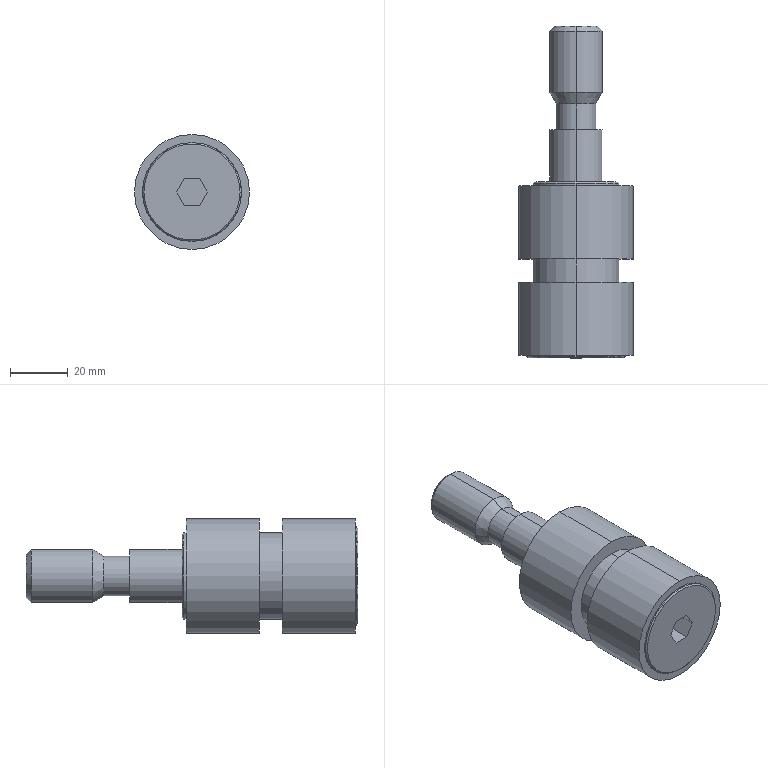Part | SolidWorks | features BaseBody 1 | 1 solid | 39 faces | box 40 x 115.385 x 40 mm | volume 83771 mm3 | cylinder 16 | plane 15 | cone 8 | commonest cylinder face diameters 18.462 x4 30 x4 40 x4 13.846 x2 34.385 x2
STEP:
#1=CARTESIAN_POINT('',(57.247,271.192,266.154));
#2=VERTEX_POINT('',#1);
#3=CARTESIAN_POINT('',(57.247,271.192,226.154));
#4=VERTEX_POINT('',#3);
#5=CARTESIAN_POINT('',(57.247,271.192,246.154));
#6=DIRECTION('',(0.,1.,0.));
#7=DIRECTION('',(0.,0.,1.));
#8=AXIS2_PLACEMENT_3D('',#5,#6,#7);
#9=CIRCLE('',#8,20.);
#10=EDGE_CURVE('',#2,#4,#9,.T.);
#11=ORIENTED_EDGE('',*,*,#10,.T.);
#12=CARTESIAN_POINT('',(57.247,296.577,226.154));
#13=VERTEX_POINT('',#12);
#14=CARTESIAN_POINT('',(57.247,270.269,226.154));
#15=DIRECTION('',(0.,1.,0.));
#16=VECTOR('',#15,1000.);
#17=LINE('',#14,#16);
#18=EDGE_CURVE('',#4,#13,#17,.T.);
#19=ORIENTED_EDGE('',*,*,#18,.T.);
#20=CARTESIAN_POINT('',(57.247,296.577,266.154));
#21=VERTEX_POINT('',#20);
#22=CARTESIAN_POINT('',(57.247,296.577,246.154));
#23=DIRECTION('',(0.,-1.,0.));
#24=DIRECTION('',(0.,0.,1.));
#25=AXIS2_PLACEMENT_3D('',#22,#23,#24);
#26=CIRCLE('',#25,20.);
#27=EDGE_CURVE('',#13,#21,#26,.T.);
#28=ORIENTED_EDGE('',*,*,#27,.T.);
#29=CARTESIAN_POINT('',(57.247,270.269,266.154));
#30=DIRECTION('',(0.,1.,0.));
#31=VECTOR('',#30,1000.);
#32=LINE('',#29,#31);
#33=EDGE_CURVE('',#2,#21,#32,.T.);
#34=ORIENTED_EDGE('',*,*,#33,.F.);
#35=EDGE_LOOP('',(#11,#19,#28,#34));
#36=FACE_OUTER_BOUND('',#35,.T.);
#37=CARTESIAN_POINT('',(57.247,270.269,246.154));
#38=DIRECTION('',(0.,1.,0.));
#39=DIRECTION('',(0.,0.,1.));
#40=AXIS2_PLACEMENT_3D('',#37,#38,#39);
#41=CYLINDRICAL_SURFACE('',#40,20.);
#42=ADVANCED_FACE('',(#36),#41,.T.);
#43=CARTESIAN_POINT('',(74.439,270.731,246.154));
#44=VERTEX_POINT('',#43);
#45=CARTESIAN_POINT('',(57.247,270.731,228.962));
#46=VERTEX_POINT('',#45);
#47=CARTESIAN_POINT('',(57.247,270.731,246.154));
#48=DIRECTION('',(0.,1.,0.));
#49=DIRECTION('',(0.,0.,1.));
#50=AXIS2_PLACEMENT_3D('',#47,#48,#49);
#51=CIRCLE('',#50,17.192);
#52=EDGE_CURVE('',#44,#46,#51,.T.);
#53=ORIENTED_EDGE('',*,*,#52,.T.);
#54=CARTESIAN_POINT('',(57.247,271.192,228.962));
#55=VERTEX_POINT('',#54);
#56=CARTESIAN_POINT('',(57.247,270.269,228.962));
#57=DIRECTION('',(0.,1.,0.));
#58=VECTOR('',#57,1000.);
#59=LINE('',#56,#58);
#60=EDGE_CURVE('',#46,#55,#59,.T.);
#61=ORIENTED_EDGE('',*,*,#60,.T.);
#62=CARTESIAN_POINT('',(57.247,271.192,263.346));
#63=VERTEX_POINT('',#62);
#64=CARTESIAN_POINT('',(57.247,271.192,246.154));
#65=DIRECTION('',(0.,-1.,0.));
#66=DIRECTION('',(0.,0.,1.));
#67=AXIS2_PLACEMENT_3D('',#64,#65,#66);
#68=CIRCLE('',#67,17.192);
#69=EDGE_CURVE('',#55,#63,#68,.T.);
#70=ORIENTED_EDGE('',*,*,#69,.T.);
#71=CARTESIAN_POINT('',(57.247,270.731,263.346));
#72=VERTEX_POINT('',#71);
#73=CARTESIAN_POINT('',(57.247,270.269,263.346));
#74=DIRECTION('',(0.,1.,0.));
#75=VECTOR('',#74,1000.);
#76=LINE('',#73,#75);
#77=EDGE_CURVE('',#72,#63,#76,.T.);
#78=ORIENTED_EDGE('',*,*,#77,.F.);
#79=CARTESIAN_POINT('',(57.247,270.731,246.154));
#80=DIRECTION('',(0.,1.,0.));
#81=DIRECTION('',(0.,0.,1.));
#82=AXIS2_PLACEMENT_3D('',#79,#80,#81);
#83=CIRCLE('',#82,17.192);
#84=EDGE_CURVE('',#72,#44,#83,.T.);
#85=ORIENTED_EDGE('',*,*,#84,.T.);
#86=EDGE_LOOP('',(#53,#61,#70,#78,#85));
#87=FACE_OUTER_BOUND('',#86,.T.);
#88=CARTESIAN_POINT('',(57.247,270.269,246.154));
#89=DIRECTION('',(0.,1.,0.));
#90=DIRECTION('',(0.,0.,1.));
#91=AXIS2_PLACEMENT_3D('',#88,#89,#90);
#92=CYLINDRICAL_SURFACE('',#91,17.192);
#93=ADVANCED_FACE('',(#87),#92,.T.);
#94=CARTESIAN_POINT('',(57.247,296.577,261.154));
#95=VERTEX_POINT('',#94);
#96=CARTESIAN_POINT('',(57.247,296.577,231.154));
#97=VERTEX_POINT('',#96);
#98=CARTESIAN_POINT('',(57.247,296.577,246.154));
#99=DIRECTION('',(0.,1.,0.));
#100=DIRECTION('',(0.,0.,1.));
#101=AXIS2_PLACEMENT_3D('',#98,#99,#100);
#102=CIRCLE('',#101,15.);
#103=EDGE_CURVE('',#95,#97,#102,.T.);
#104=ORIENTED_EDGE('',*,*,#103,.T.);
#105=CARTESIAN_POINT('',(57.247,304.654,231.154));
#106=VERTEX_POINT('',#105);
#107=CARTESIAN_POINT('',(57.247,270.269,231.154));
#108=DIRECTION('',(0.,1.,0.));
#109=VECTOR('',#108,1000.);
#110=LINE('',#107,#109);
#111=EDGE_CURVE('',#97,#106,#110,.T.);
#112=ORIENTED_EDGE('',*,*,#111,.T.);
#113=CARTESIAN_POINT('',(57.247,304.654,261.154));
#114=VERTEX_POINT('',#113);
#115=CARTESIAN_POINT('',(57.247,304.654,246.154));
#116=DIRECTION('',(0.,-1.,0.));
#117=DIRECTION('',(0.,0.,1.));
#118=AXIS2_PLACEMENT_3D('',#115,#116,#117);
#119=CIRCLE('',#118,15.);
#120=EDGE_CURVE('',#106,#114,#119,.T.);
#121=ORIENTED_EDGE('',*,*,#120,.T.);
#122=CARTESIAN_POINT('',(57.247,270.269,261.154));
#123=DIRECTION('',(0.,1.,0.));
#124=VECTOR('',#123,1000.);
#125=LINE('',#122,#124);
#126=EDGE_CURVE('',#95,#114,#125,.T.);
#127=ORIENTED_EDGE('',*,*,#126,.F.);
#128=EDGE_LOOP('',(#104,#112,#121,#127));
#129=FACE_OUTER_BOUND('',#128,.T.);
#130=CARTESIAN_POINT('',(57.247,270.269,246.154));
#131=DIRECTION('',(0.,1.,0.));
#132=DIRECTION('',(0.,0.,1.));
#133=AXIS2_PLACEMENT_3D('',#130,#131,#132);
#134=CYLINDRICAL_SURFACE('',#133,15.);
#135=ADVANCED_FACE('',(#129),#134,.T.);
#136=CARTESIAN_POINT('',(40.516,270.269,246.154));
#137=VERTEX_POINT('',#136);
#138=CARTESIAN_POINT('',(73.977,270.269,246.154));
#139=VERTEX_POINT('',#138);
#140=CARTESIAN_POINT('',(57.247,270.269,246.154));
#141=DIRECTION('',(0.,1.,0.));
#142=DIRECTION('',(-1.,0.,0.));
#143=AXIS2_PLACEMENT_3D('',#140,#141,#142);
#144=CIRCLE('',#143,16.731);
#145=EDGE_CURVE('',#137,#139,#144,.T.);
#146=ORIENTED_EDGE('',*,*,#145,.T.);
#147=CARTESIAN_POINT('',(74.439,270.731,246.154));
#148=DIRECTION('',(0.7071,0.7071,0.));
#149=VECTOR('',#148,1000.);
#150=LINE('',#147,#149);
#151=EDGE_CURVE('',#139,#44,#150,.T.);
#152=ORIENTED_EDGE('',*,*,#151,.T.);
#153=ORIENTED_EDGE('',*,*,#84,.F.);
#154=CARTESIAN_POINT('',(40.054,270.731,246.154));
#155=VERTEX_POINT('',#154);
#156=CARTESIAN_POINT('',(57.247,270.731,246.154));
#157=DIRECTION('',(0.,1.,0.));
#158=DIRECTION('',(0.,0.,1.));
#159=AXIS2_PLACEMENT_3D('',#156,#157,#158);
#160=CIRCLE('',#159,17.192);
#161=EDGE_CURVE('',#155,#72,#160,.T.);
#162=ORIENTED_EDGE('',*,*,#161,.F.);
#163=CARTESIAN_POINT('',(40.054,270.731,246.154));
#164=DIRECTION('',(-0.7071,0.7071,0.));
#165=VECTOR('',#164,1000.);
#166=LINE('',#163,#165);
#167=EDGE_CURVE('',#137,#155,#166,.T.);
#168=ORIENTED_EDGE('',*,*,#167,.F.);
#169=EDGE_LOOP('',(#146,#152,#153,#162,#168));
#170=FACE_OUTER_BOUND('',#169,.T.);
#171=CARTESIAN_POINT('',(57.247,270.731,246.154));
#172=DIRECTION('',(0.,1.,0.));
#173=DIRECTION('',(-1.,0.,0.));
#174=AXIS2_PLACEMENT_3D('',#171,#172,#173);
#175=CONICAL_SURFACE('',#174,17.192,0.7854);
#176=ADVANCED_FACE('',(#170),#175,.T.);
#177=CARTESIAN_POINT('',(57.247,304.654,266.154));
#178=VERTEX_POINT('',#177);
#179=CARTESIAN_POINT('',(57.247,304.654,226.154));
#180=VERTEX_POINT('',#179);
#181=CARTESIAN_POINT('',(57.247,304.654,246.154));
#182=DIRECTION('',(0.,1.,0.));
#183=DIRECTION('',(0.,0.,1.));
#184=AXIS2_PLACEMENT_3D('',#181,#182,#183);
#185=CIRCLE('',#184,20.);
#186=EDGE_CURVE('',#178,#180,#185,.T.);
#187=ORIENTED_EDGE('',*,*,#186,.T.);
#188=CARTESIAN_POINT('',(57.247,330.038,226.154));
#189=VERTEX_POINT('',#188);
#190=CARTESIAN_POINT('',(57.247,270.269,226.154));
#191=DIRECTION('',(0.,1.,0.));
#192=VECTOR('',#191,1000.);
#193=LINE('',#190,#192);
#194=EDGE_CURVE('',#180,#189,#193,.T.);
#195=ORIENTED_EDGE('',*,*,#194,.T.);
#196=CARTESIAN_POINT('',(57.247,330.038,266.154));
#197=VERTEX_POINT('',#196);
#198=CARTESIAN_POINT('',(57.247,330.038,246.154));
#199=DIRECTION('',(0.,-1.,0.));
#200=DIRECTION('',(0.,0.,1.));
#201=AXIS2_PLACEMENT_3D('',#198,#199,#200);
#202=CIRCLE('',#201,20.);
#203=EDGE_CURVE('',#189,#197,#202,.T.);
#204=ORIENTED_EDGE('',*,*,#203,.T.);
#205=CARTESIAN_POINT('',(57.247,270.269,266.154));
#206=DIRECTION('',(0.,1.,0.));
#207=VECTOR('',#206,1000.);
#208=LINE('',#205,#207);
#209=EDGE_CURVE('',#178,#197,#208,.T.);
#210=ORIENTED_EDGE('',*,*,#209,.F.);
#211=EDGE_LOOP('',(#187,#195,#204,#210));
#212=FACE_OUTER_BOUND('',#211,.T.);
#213=CARTESIAN_POINT('',(57.247,270.269,246.154));
#214=DIRECTION('',(0.,1.,0.));
#215=DIRECTION('',(0.,0.,1.));
#216=AXIS2_PLACEMENT_3D('',#213,#214,#215);
#217=CYLINDRICAL_SURFACE('',#216,20.);
#218=ADVANCED_FACE('',(#212),#217,.T.);
#219=CARTESIAN_POINT('',(57.247,330.038,261.154));
#220=VERTEX_POINT('',#219);
#221=CARTESIAN_POINT('',(57.247,330.038,231.154));
#222=VERTEX_POINT('',#221);
#223=CARTESIAN_POINT('',(57.247,330.038,246.154));
#224=DIRECTION('',(0.,1.,0.));
#225=DIRECTION('',(0.,0.,1.));
#226=AXIS2_PLACEMENT_3D('',#223,#224,#225);
#227=CIRCLE('',#226,15.);
#228=EDGE_CURVE('',#220,#222,#227,.T.);
#229=ORIENTED_EDGE('',*,*,#228,.T.);
#230=CARTESIAN_POINT('',(57.247,330.962,231.154));
#231=VERTEX_POINT('',#230);
#232=CARTESIAN_POINT('',(57.247,270.269,231.154));
#233=DIRECTION('',(0.,1.,0.));
#234=VECTOR('',#233,1000.);
#235=LINE('',#232,#234);
#236=EDGE_CURVE('',#222,#231,#235,.T.);
#237=ORIENTED_EDGE('',*,*,#236,.T.);
#238=CARTESIAN_POINT('',(57.247,330.962,261.154));
#239=VERTEX_POINT('',#238);
#240=CARTESIAN_POINT('',(57.247,330.962,246.154));
#241=DIRECTION('',(0.,-1.,0.));
#242=DIRECTION('',(0.,0.,1.));
#243=AXIS2_PLACEMENT_3D('',#240,#241,#242);
#244=CIRCLE('',#243,15.);
#245=EDGE_CURVE('',#231,#239,#244,.T.);
#246=ORIENTED_EDGE('',*,*,#245,.T.);
#247=CARTESIAN_POINT('',(57.247,270.269,261.154));
#248=DIRECTION('',(0.,1.,0.));
#249=VECTOR('',#248,1000.);
#250=LINE('',#247,#249);
#251=EDGE_CURVE('',#220,#239,#250,.T.);
#252=ORIENTED_EDGE('',*,*,#251,.F.);
#253=EDGE_LOOP('',(#229,#237,#246,#252));
#254=FACE_OUTER_BOUND('',#253,.T.);
#255=CARTESIAN_POINT('',(57.247,270.269,246.154));
#256=DIRECTION('',(0.,1.,0.));
#257=DIRECTION('',(0.,0.,1.));
#258=AXIS2_PLACEMENT_3D('',#255,#256,#257);
#259=CYLINDRICAL_SURFACE('',#258,15.);
#260=ADVANCED_FACE('',(#254),#259,.T.);
#261=CARTESIAN_POINT('',(57.247,331.423,231.615));
#262=VERTEX_POINT('',#261);
#263=CARTESIAN_POINT('',(57.247,331.423,260.692));
#264=VERTEX_POINT('',#263);
#265=CARTESIAN_POINT('',(57.247,331.423,246.154));
#266=DIRECTION('',(0.,-1.,0.));
#267=DIRECTION('',(0.,0.,-1.));
#268=AXIS2_PLACEMENT_3D('',#265,#266,#267);
#269=CIRCLE('',#268,14.538);
#270=EDGE_CURVE('',#262,#264,#269,.T.);
#271=ORIENTED_EDGE('',*,*,#270,.T.);
#272=CARTESIAN_POINT('',(57.247,330.962,261.154));
#273=DIRECTION('',(0.,-0.7071,0.7071));
#274=VECTOR('',#273,1000.);
#275=LINE('',#272,#274);
#276=EDGE_CURVE('',#264,#239,#275,.T.);
#277=ORIENTED_EDGE('',*,*,#276,.T.);
#278=ORIENTED_EDGE('',*,*,#245,.F.);
#279=CARTESIAN_POINT('',(57.247,330.962,231.154));
#280=DIRECTION('',(0.,-0.7071,-0.7071));
#281=VECTOR('',#280,1000.);
#282=LINE('',#279,#281);
#283=EDGE_CURVE('',#262,#231,#282,.T.);
#284=ORIENTED_EDGE('',*,*,#283,.F.);
#285=EDGE_LOOP('',(#271,#277,#278,#284));
#286=FACE_OUTER_BOUND('',#285,.T.);
#287=CARTESIAN_POINT('',(57.247,330.962,246.154));
#288=DIRECTION('',(0.,-1.,0.));
#289=DIRECTION('',(0.,0.,-1.));
#290=AXIS2_PLACEMENT_3D('',#287,#288,#289);
#291=CONICAL_SURFACE('',#290,15.,0.7854);
#292=ADVANCED_FACE('',(#286),#291,.T.);
#293=CARTESIAN_POINT('',(57.247,331.423,255.385));
#294=VERTEX_POINT('',#293);
#295=CARTESIAN_POINT('',(57.247,331.423,236.923));
#296=VERTEX_POINT('',#295);
#297=CARTESIAN_POINT('',(57.247,331.423,246.154));
#298=DIRECTION('',(0.,1.,0.));
#299=DIRECTION('',(0.,0.,1.));
#300=AXIS2_PLACEMENT_3D('',#297,#298,#299);
#301=CIRCLE('',#300,9.231);
#302=EDGE_CURVE('',#294,#296,#301,.T.);
#303=ORIENTED_EDGE('',*,*,#302,.T.);
#304=CARTESIAN_POINT('',(57.247,349.556,236.923));
#305=VERTEX_POINT('',#304);
#306=CARTESIAN_POINT('',(57.247,270.269,236.923));
#307=DIRECTION('',(0.,1.,0.));
#308=VECTOR('',#307,1000.);
#309=LINE('',#306,#308);
#310=EDGE_CURVE('',#296,#305,#309,.T.);
#311=ORIENTED_EDGE('',*,*,#310,.T.);
#312=CARTESIAN_POINT('',(57.247,349.556,255.385));
#313=VERTEX_POINT('',#312);
#314=CARTESIAN_POINT('',(57.247,349.556,246.154));
#315=DIRECTION('',(0.,-1.,0.));
#316=DIRECTION('',(0.,0.,1.));
#317=AXIS2_PLACEMENT_3D('',#314,#315,#316);
#318=CIRCLE('',#317,9.231);
#319=EDGE_CURVE('',#305,#313,#318,.T.);
#320=ORIENTED_EDGE('',*,*,#319,.T.);
#321=CARTESIAN_POINT('',(57.247,270.269,255.385));
#322=DIRECTION('',(0.,1.,0.));
#323=VECTOR('',#322,1000.);
#324=LINE('',#321,#323);
#325=EDGE_CURVE('',#294,#313,#324,.T.);
#326=ORIENTED_EDGE('',*,*,#325,.F.);
#327=EDGE_LOOP('',(#303,#311,#320,#326));
#328=FACE_OUTER_BOUND('',#327,.T.);
#329=CARTESIAN_POINT('',(57.247,270.269,246.154));
#330=DIRECTION('',(0.,1.,0.));
#331=DIRECTION('',(0.,0.,1.));
#332=AXIS2_PLACEMENT_3D('',#329,#330,#331);
#333=CYLINDRICAL_SURFACE('',#332,9.231);
#334=ADVANCED_FACE('',(#328),#333,.T.);
#335=CARTESIAN_POINT('',(57.247,349.556,253.077));
#336=VERTEX_POINT('',#335);
#337=CARTESIAN_POINT('',(57.247,349.556,239.231));
#338=VERTEX_POINT('',#337);
#339=CARTESIAN_POINT('',(57.247,349.556,246.154));
#340=DIRECTION('',(0.,1.,0.));
#341=DIRECTION('',(0.,0.,1.));
#342=AXIS2_PLACEMENT_3D('',#339,#340,#341);
#343=CIRCLE('',#342,6.923);
#344=EDGE_CURVE('',#336,#338,#343,.T.);
#345=ORIENTED_EDGE('',*,*,#344,.T.);
#346=CARTESIAN_POINT('',(57.247,358.58,239.231));
#347=VERTEX_POINT('',#346);
#348=CARTESIAN_POINT('',(57.247,270.269,239.231));
#349=DIRECTION('',(0.,1.,0.));
#350=VECTOR('',#349,1000.);
#351=LINE('',#348,#350);
#352=EDGE_CURVE('',#338,#347,#351,.T.);
#353=ORIENTED_EDGE('',*,*,#352,.T.);
#354=CARTESIAN_POINT('',(57.247,358.58,253.077));
#355=VERTEX_POINT('',#354);
#356=CARTESIAN_POINT('',(57.247,358.58,246.154));
#357=DIRECTION('',(0.,-1.,0.));
#358=DIRECTION('',(0.,0.,1.));
#359=AXIS2_PLACEMENT_3D('',#356,#357,#358);
#360=CIRCLE('',#359,6.923);
#361=EDGE_CURVE('',#347,#355,#360,.T.);
#362=ORIENTED_EDGE('',*,*,#361,.T.);
#363=CARTESIAN_POINT('',(57.247,270.269,253.077));
#364=DIRECTION('',(0.,1.,0.));
#365=VECTOR('',#364,1000.);
#366=LINE('',#363,#365);
#367=EDGE_CURVE('',#336,#355,#366,.T.);
#368=ORIENTED_EDGE('',*,*,#367,.F.);
#369=EDGE_LOOP('',(#345,#353,#362,#368));
#370=FACE_OUTER_BOUND('',#369,.T.);
#371=CARTESIAN_POINT('',(57.247,270.269,246.154));
#372=DIRECTION('',(0.,1.,0.));
#373=DIRECTION('',(0.,0.,1.));
#374=AXIS2_PLACEMENT_3D('',#371,#372,#373);
#375=CYLINDRICAL_SURFACE('',#374,6.923);
#376=ADVANCED_FACE('',(#370),#375,.T.);
#377=ORIENTED_EDGE('',*,*,#361,.F.);
#378=CARTESIAN_POINT('',(57.247,362.577,236.923));
#379=VERTEX_POINT('',#378);
#380=CARTESIAN_POINT('',(57.247,362.577,236.923));
#381=DIRECTION('',(0.,0.866,-0.5));
#382=VECTOR('',#381,1000.);
#383=LINE('',#380,#382);
#384=EDGE_CURVE('',#347,#379,#383,.T.);
#385=ORIENTED_EDGE('',*,*,#384,.T.);
#386=CARTESIAN_POINT('',(57.247,362.577,255.385));
#387=VERTEX_POINT('',#386);
#388=CARTESIAN_POINT('',(57.247,362.577,246.154));
#389=DIRECTION('',(0.,-1.,0.));
#390=DIRECTION('',(-1.,0.,0.));
#391=AXIS2_PLACEMENT_3D('',#388,#389,#390);
#392=CIRCLE('',#391,9.231);
#393=EDGE_CURVE('',#379,#387,#392,.T.);
#394=ORIENTED_EDGE('',*,*,#393,.T.);
#395=CARTESIAN_POINT('',(57.247,362.577,255.385));
#396=DIRECTION('',(0.,0.866,0.5));
#397=VECTOR('',#396,1000.);
#398=LINE('',#395,#397);
#399=EDGE_CURVE('',#355,#387,#398,.T.);
#400=ORIENTED_EDGE('',*,*,#399,.F.);
#401=EDGE_LOOP('',(#377,#385,#394,#400));
#402=FACE_OUTER_BOUND('',#401,.T.);
#403=CARTESIAN_POINT('',(57.247,362.577,246.154));
#404=DIRECTION('',(0.,1.,0.));
#405=DIRECTION('',(0.,0.,1.));
#406=AXIS2_PLACEMENT_3D('',#403,#404,#405);
#407=CONICAL_SURFACE('',#406,9.231,0.5236);
#408=ADVANCED_FACE('',(#402),#407,.T.);
#409=ORIENTED_EDGE('',*,*,#393,.F.);
#410=CARTESIAN_POINT('',(57.247,383.884,236.923));
#411=VERTEX_POINT('',#410);
#412=CARTESIAN_POINT('',(57.247,270.269,236.923));
#413=DIRECTION('',(0.,1.,0.));
#414=VECTOR('',#413,1000.);
#415=LINE('',#412,#414);
#416=EDGE_CURVE('',#379,#411,#415,.T.);
#417=ORIENTED_EDGE('',*,*,#416,.T.);
#418=CARTESIAN_POINT('',(57.247,383.884,255.385));
#419=VERTEX_POINT('',#418);
#420=CARTESIAN_POINT('',(57.247,383.884,246.154));
#421=DIRECTION('',(0.,-1.,0.));
#422=DIRECTION('',(0.,0.,1.));
#423=AXIS2_PLACEMENT_3D('',#420,#421,#422);
#424=CIRCLE('',#423,9.231);
#425=EDGE_CURVE('',#411,#419,#424,.T.);
#426=ORIENTED_EDGE('',*,*,#425,.T.);
#427=CARTESIAN_POINT('',(57.247,270.269,255.385));
#428=DIRECTION('',(0.,1.,0.));
#429=VECTOR('',#428,1000.);
#430=LINE('',#427,#429);
#431=EDGE_CURVE('',#387,#419,#430,.T.);
#432=ORIENTED_EDGE('',*,*,#431,.F.);
#433=EDGE_LOOP('',(#409,#417,#426,#432));
#434=FACE_OUTER_BOUND('',#433,.T.);
#435=CARTESIAN_POINT('',(57.247,270.269,246.154));
#436=DIRECTION('',(0.,1.,0.));
#437=DIRECTION('',(0.,0.,1.));
#438=AXIS2_PLACEMENT_3D('',#435,#436,#437);
#439=CYLINDRICAL_SURFACE('',#438,9.231);
#440=ADVANCED_FACE('',(#434),#439,.T.);
#441=CARTESIAN_POINT('',(57.247,385.654,238.693));
#442=VERTEX_POINT('',#441);
#443=CARTESIAN_POINT('',(57.247,385.654,253.615));
#444=VERTEX_POINT('',#443);
#445=CARTESIAN_POINT('',(57.247,385.654,246.154));
#446=DIRECTION('',(0.,-1.,0.));
#447=DIRECTION('',(0.,0.,-1.));
#448=AXIS2_PLACEMENT_3D('',#445,#446,#447);
#449=CIRCLE('',#448,7.461);
#450=EDGE_CURVE('',#442,#444,#449,.T.);
#451=ORIENTED_EDGE('',*,*,#450,.T.);
#452=CARTESIAN_POINT('',(57.247,383.884,255.385));
#453=DIRECTION('',(0.,-0.7071,0.7071));
#454=VECTOR('',#453,1000.);
#455=LINE('',#452,#454);
#456=EDGE_CURVE('',#444,#419,#455,.T.);
#457=ORIENTED_EDGE('',*,*,#456,.T.);
#458=ORIENTED_EDGE('',*,*,#425,.F.);
#459=CARTESIAN_POINT('',(57.247,383.884,236.923));
#460=DIRECTION('',(0.,-0.7071,-0.7071));
#461=VECTOR('',#460,1000.);
#462=LINE('',#459,#461);
#463=EDGE_CURVE('',#442,#411,#462,.T.);
#464=ORIENTED_EDGE('',*,*,#463,.F.);
#465=EDGE_LOOP('',(#451,#457,#458,#464));
#466=FACE_OUTER_BOUND('',#465,.T.);
#467=CARTESIAN_POINT('',(57.247,383.884,246.154));
#468=DIRECTION('',(0.,-1.,0.));
#469=DIRECTION('',(0.,0.,-1.));
#470=AXIS2_PLACEMENT_3D('',#467,#468,#469);
#471=CONICAL_SURFACE('',#470,9.231,0.7854);
#472=ADVANCED_FACE('',(#466),#471,.T.);
#473=ORIENTED_EDGE('',*,*,#18,.F.);
#474=CARTESIAN_POINT('',(57.247,271.192,246.154));
#475=DIRECTION('',(0.,1.,0.));
#476=DIRECTION('',(0.,0.,1.));
#477=AXIS2_PLACEMENT_3D('',#474,#475,#476);
#478=CIRCLE('',#477,20.);
#479=EDGE_CURVE('',#4,#2,#478,.T.);
#480=ORIENTED_EDGE('',*,*,#479,.T.);
#481=ORIENTED_EDGE('',*,*,#33,.T.);
#482=CARTESIAN_POINT('',(57.247,296.577,246.154));
#483=DIRECTION('',(0.,-1.,0.));
#484=DIRECTION('',(0.,0.,1.));
#485=AXIS2_PLACEMENT_3D('',#482,#483,#484);
#486=CIRCLE('',#485,20.);
#487=EDGE_CURVE('',#21,#13,#486,.T.);
#488=ORIENTED_EDGE('',*,*,#487,.T.);
#489=EDGE_LOOP('',(#473,#480,#481,#488));
#490=FACE_OUTER_BOUND('',#489,.T.);
#491=CARTESIAN_POINT('',(57.247,270.269,246.154));
#492=DIRECTION('',(0.,1.,0.));
#493=DIRECTION('',(0.,0.,1.));
#494=AXIS2_PLACEMENT_3D('',#491,#492,#493);
#495=CYLINDRICAL_SURFACE('',#494,20.);
#496=ADVANCED_FACE('',(#490),#495,.T.);
#497=CARTESIAN_POINT('',(57.247,271.192,246.154));
#498=DIRECTION('',(0.,-1.,0.));
#499=DIRECTION('',(0.,0.,1.));
#500=AXIS2_PLACEMENT_3D('',#497,#498,#499);
#501=CIRCLE('',#500,17.192);
#502=EDGE_CURVE('',#63,#55,#501,.T.);
#503=ORIENTED_EDGE('',*,*,#502,.F.);
#504=ORIENTED_EDGE('',*,*,#69,.F.);
#505=EDGE_LOOP('',(#503,#504));
#506=FACE_BOUND('',#505,.T.);
#507=ORIENTED_EDGE('',*,*,#10,.F.);
#508=ORIENTED_EDGE('',*,*,#479,.F.);
#509=EDGE_LOOP('',(#507,#508));
#510=FACE_OUTER_BOUND('',#509,.T.);
#511=CARTESIAN_POINT('',(57.247,271.192,224.923));
#512=DIRECTION('',(0.,1.,0.));
#513=DIRECTION('',(0.,0.,1.));
#514=AXIS2_PLACEMENT_3D('',#511,#512,#513);
#515=PLANE('',#514);
#516=ADVANCED_FACE('',(#506,#510),#515,.F.);
#517=ORIENTED_EDGE('',*,*,#103,.F.);
#518=CARTESIAN_POINT('',(57.247,296.577,246.154));
#519=DIRECTION('',(0.,1.,0.));
#520=DIRECTION('',(0.,0.,1.));
#521=AXIS2_PLACEMENT_3D('',#518,#519,#520);
#522=CIRCLE('',#521,15.);
#523=EDGE_CURVE('',#97,#95,#522,.T.);
#524=ORIENTED_EDGE('',*,*,#523,.F.);
#525=EDGE_LOOP('',(#517,#524));
#526=FACE_BOUND('',#525,.T.);
#527=ORIENTED_EDGE('',*,*,#487,.F.);
#528=ORIENTED_EDGE('',*,*,#27,.F.);
#529=EDGE_LOOP('',(#527,#528));
#530=FACE_OUTER_BOUND('',#529,.T.);
#531=CARTESIAN_POINT('',(57.247,296.577,231.154));
#532=DIRECTION('',(0.,-1.,0.));
#533=DIRECTION('',(0.,0.,-1.));
#534=AXIS2_PLACEMENT_3D('',#531,#532,#533);
#535=PLANE('',#534);
#536=ADVANCED_FACE('',(#526,#530),#535,.F.);
#537=ORIENTED_EDGE('',*,*,#60,.F.);
#538=CARTESIAN_POINT('',(57.247,270.731,246.154));
#539=DIRECTION('',(0.,1.,0.));
#540=DIRECTION('',(0.,0.,1.));
#541=AXIS2_PLACEMENT_3D('',#538,#539,#540);
#542=CIRCLE('',#541,17.192);
#543=EDGE_CURVE('',#46,#155,#542,.T.);
#544=ORIENTED_EDGE('',*,*,#543,.T.);
#545=ORIENTED_EDGE('',*,*,#161,.T.);
#546=ORIENTED_EDGE('',*,*,#77,.T.);
#547=ORIENTED_EDGE('',*,*,#502,.T.);
#548=EDGE_LOOP('',(#537,#544,#545,#546,#547));
#549=FACE_OUTER_BOUND('',#548,.T.);
#550=CARTESIAN_POINT('',(57.247,270.269,246.154));
#551=DIRECTION('',(0.,1.,0.));
#552=DIRECTION('',(0.,0.,1.));
#553=AXIS2_PLACEMENT_3D('',#550,#551,#552);
#554=CYLINDRICAL_SURFACE('',#553,17.192);
#555=ADVANCED_FACE('',(#549),#554,.T.);
#556=ORIENTED_EDGE('',*,*,#111,.F.);
#557=ORIENTED_EDGE('',*,*,#523,.T.);
#558=ORIENTED_EDGE('',*,*,#126,.T.);
#559=CARTESIAN_POINT('',(57.247,304.654,246.154));
#560=DIRECTION('',(0.,-1.,0.));
#561=DIRECTION('',(0.,0.,1.));
#562=AXIS2_PLACEMENT_3D('',#559,#560,#561);
#563=CIRCLE('',#562,15.);
#564=EDGE_CURVE('',#114,#106,#563,.T.);
#565=ORIENTED_EDGE('',*,*,#564,.T.);
#566=EDGE_LOOP('',(#556,#557,#558,#565));
#567=FACE_OUTER_BOUND('',#566,.T.);
#568=CARTESIAN_POINT('',(57.247,270.269,246.154));
#569=DIRECTION('',(0.,1.,0.));
#570=DIRECTION('',(0.,0.,1.));
#571=AXIS2_PLACEMENT_3D('',#568,#569,#570);
#572=CYLINDRICAL_SURFACE('',#571,15.);
#573=ADVANCED_FACE('',(#567),#572,.T.);
#574=ORIENTED_EDGE('',*,*,#151,.F.);
#575=CARTESIAN_POINT('',(57.247,270.269,246.154));
#576=DIRECTION('',(0.,1.,0.));
#577=DIRECTION('',(-1.,0.,0.));
#578=AXIS2_PLACEMENT_3D('',#575,#576,#577);
#579=CIRCLE('',#578,16.731);
#580=EDGE_CURVE('',#139,#137,#579,.T.);
#581=ORIENTED_EDGE('',*,*,#580,.T.);
#582=ORIENTED_EDGE('',*,*,#167,.T.);
#583=ORIENTED_EDGE('',*,*,#543,.F.);
#584=ORIENTED_EDGE('',*,*,#52,.F.);
#585=EDGE_LOOP('',(#574,#581,#582,#583,#584));
#586=FACE_OUTER_BOUND('',#585,.T.);
#587=CARTESIAN_POINT('',(57.247,270.731,246.154));
#588=DIRECTION('',(0.,1.,0.));
#589=DIRECTION('',(-1.,0.,0.));
#590=AXIS2_PLACEMENT_3D('',#587,#588,#589);
#591=CONICAL_SURFACE('',#590,17.192,0.7854);
#592=ADVANCED_FACE('',(#586),#591,.T.);
#593=ORIENTED_EDGE('',*,*,#564,.F.);
#594=ORIENTED_EDGE('',*,*,#120,.F.);
#595=EDGE_LOOP('',(#593,#594));
#596=FACE_BOUND('',#595,.T.);
#597=ORIENTED_EDGE('',*,*,#186,.F.);
#598=CARTESIAN_POINT('',(57.247,304.654,246.154));
#599=DIRECTION('',(0.,1.,0.));
#600=DIRECTION('',(0.,0.,1.));
#601=AXIS2_PLACEMENT_3D('',#598,#599,#600);
#602=CIRCLE('',#601,20.);
#603=EDGE_CURVE('',#180,#178,#602,.T.);
#604=ORIENTED_EDGE('',*,*,#603,.F.);
#605=EDGE_LOOP('',(#597,#604));
#606=FACE_OUTER_BOUND('',#605,.T.);
#607=CARTESIAN_POINT('',(57.247,304.654,224.692));
#608=DIRECTION('',(0.,1.,0.));
#609=DIRECTION('',(0.,0.,1.));
#610=AXIS2_PLACEMENT_3D('',#607,#608,#609);
#611=PLANE('',#610);
#612=ADVANCED_FACE('',(#596,#606),#611,.F.);
#613=CARTESIAN_POINT('',(59.911,270.269,250.769));
#614=VERTEX_POINT('',#613);
#615=CARTESIAN_POINT('',(54.582,270.269,250.769));
#616=VERTEX_POINT('',#615);
#617=CARTESIAN_POINT('',(57.247,270.269,250.769));
#618=DIRECTION('',(-1.,0.,0.));
#619=VECTOR('',#618,1000.);
#620=LINE('',#617,#619);
#621=EDGE_CURVE('',#614,#616,#620,.T.);
#622=ORIENTED_EDGE('',*,*,#621,.F.);
#623=CARTESIAN_POINT('',(62.576,270.269,246.154));
#624=VERTEX_POINT('',#623);
#625=CARTESIAN_POINT('',(62.576,270.269,246.154));
#626=DIRECTION('',(-0.5,0.,0.866));
#627=VECTOR('',#626,1000.);
#628=LINE('',#625,#627);
#629=EDGE_CURVE('',#624,#614,#628,.T.);
#630=ORIENTED_EDGE('',*,*,#629,.F.);
#631=CARTESIAN_POINT('',(59.911,270.269,241.538));
#632=VERTEX_POINT('',#631);
#633=CARTESIAN_POINT('',(59.911,270.269,241.538));
#634=DIRECTION('',(0.5,0.,0.866));
#635=VECTOR('',#634,1000.);
#636=LINE('',#633,#635);
#637=EDGE_CURVE('',#632,#624,#636,.T.);
#638=ORIENTED_EDGE('',*,*,#637,.F.);
#639=CARTESIAN_POINT('',(54.582,270.269,241.538));
#640=VERTEX_POINT('',#639);
#641=CARTESIAN_POINT('',(57.247,270.269,241.538));
#642=DIRECTION('',(1.,0.,0.));
#643=VECTOR('',#642,1000.);
#644=LINE('',#641,#643);
#645=EDGE_CURVE('',#640,#632,#644,.T.);
#646=ORIENTED_EDGE('',*,*,#645,.F.);
#647=CARTESIAN_POINT('',(51.917,270.269,246.154));
#648=VERTEX_POINT('',#647);
#649=CARTESIAN_POINT('',(51.917,270.269,246.154));
#650=DIRECTION('',(0.5,0.,-0.866));
#651=VECTOR('',#650,1000.);
#652=LINE('',#649,#651);
#653=EDGE_CURVE('',#648,#640,#652,.T.);
#654=ORIENTED_EDGE('',*,*,#653,.F.);
#655=CARTESIAN_POINT('',(54.582,270.269,250.769));
#656=DIRECTION('',(-0.5,0.,-0.866));
#657=VECTOR('',#656,1000.);
#658=LINE('',#655,#657);
#659=EDGE_CURVE('',#616,#648,#658,.T.);
#660=ORIENTED_EDGE('',*,*,#659,.F.);
#661=EDGE_LOOP('',(#622,#630,#638,#646,#654,#660));
#662=FACE_BOUND('',#661,.T.);
#663=ORIENTED_EDGE('',*,*,#145,.F.);
#664=ORIENTED_EDGE('',*,*,#580,.F.);
#665=EDGE_LOOP('',(#663,#664));
#666=FACE_OUTER_BOUND('',#665,.T.);
#667=CARTESIAN_POINT('',(57.247,270.269,229.423));
#668=DIRECTION('',(0.,1.,0.));
#669=DIRECTION('',(0.,0.,1.));
#670=AXIS2_PLACEMENT_3D('',#667,#668,#669);
#671=PLANE('',#670);
#672=ADVANCED_FACE('',(#662,#666),#671,.F.);
#673=ORIENTED_EDGE('',*,*,#194,.F.);
#674=ORIENTED_EDGE('',*,*,#603,.T.);
#675=ORIENTED_EDGE('',*,*,#209,.T.);
#676=CARTESIAN_POINT('',(57.247,330.038,246.154));
#677=DIRECTION('',(0.,-1.,0.));
#678=DIRECTION('',(0.,0.,1.));
#679=AXIS2_PLACEMENT_3D('',#676,#677,#678);
#680=CIRCLE('',#679,20.);
#681=EDGE_CURVE('',#197,#189,#680,.T.);
#682=ORIENTED_EDGE('',*,*,#681,.T.);
#683=EDGE_LOOP('',(#673,#674,#675,#682));
#684=FACE_OUTER_BOUND('',#683,.T.);
#685=CARTESIAN_POINT('',(57.247,270.269,246.154));
#686=DIRECTION('',(0.,1.,0.));
#687=DIRECTION('',(0.,0.,1.));
#688=AXIS2_PLACEMENT_3D('',#685,#686,#687);
#689=CYLINDRICAL_SURFACE('',#688,20.);
#690=ADVANCED_FACE('',(#684),#689,.T.);
#691=CARTESIAN_POINT('',(51.917,279.5,246.154));
#692=VERTEX_POINT('',#691);
#693=CARTESIAN_POINT('',(51.917,261.038,246.154));
#694=DIRECTION('',(0.,1.,0.));
#695=VECTOR('',#694,1000.);
#696=LINE('',#693,#695);
#697=EDGE_CURVE('',#648,#692,#696,.T.);
#698=ORIENTED_EDGE('',*,*,#697,.T.);
#699=CARTESIAN_POINT('',(54.582,279.5,250.769));
#700=VERTEX_POINT('',#699);
#701=CARTESIAN_POINT('',(54.582,279.5,250.769));
#702=DIRECTION('',(0.5,0.,0.866));
#703=VECTOR('',#702,1000.);
#704=LINE('',#701,#703);
#705=EDGE_CURVE('',#692,#700,#704,.T.);
#706=ORIENTED_EDGE('',*,*,#705,.T.);
#707=CARTESIAN_POINT('',(54.582,261.038,250.769));
#708=DIRECTION('',(0.,-1.,0.));
#709=VECTOR('',#708,1000.);
#710=LINE('',#707,#709);
#711=EDGE_CURVE('',#700,#616,#710,.T.);
#712=ORIENTED_EDGE('',*,*,#711,.T.);
#713=ORIENTED_EDGE('',*,*,#659,.T.);
#714=EDGE_LOOP('',(#698,#706,#712,#713));
#715=FACE_OUTER_BOUND('',#714,.T.);
#716=CARTESIAN_POINT('',(54.582,261.038,250.769));
#717=DIRECTION('',(0.866,0.,-0.5));
#718=DIRECTION('',(-0.5,0.,-0.866));
#719=AXIS2_PLACEMENT_3D('',#716,#717,#718);
#720=PLANE('',#719);
#721=ADVANCED_FACE('',(#715),#720,.T.);
#722=ORIENTED_EDGE('',*,*,#711,.F.);
#723=CARTESIAN_POINT('',(59.911,279.5,250.769));
#724=VERTEX_POINT('',#723);
#725=CARTESIAN_POINT('',(59.911,279.5,250.769));
#726=DIRECTION('',(1.,0.,0.));
#727=VECTOR('',#726,1000.);
#728=LINE('',#725,#727);
#729=EDGE_CURVE('',#700,#724,#728,.T.);
#730=ORIENTED_EDGE('',*,*,#729,.T.);
#731=CARTESIAN_POINT('',(59.911,261.038,250.769));
#732=DIRECTION('',(0.,-1.,0.));
#733=VECTOR('',#732,1000.);
#734=LINE('',#731,#733);
#735=EDGE_CURVE('',#724,#614,#734,.T.);
#736=ORIENTED_EDGE('',*,*,#735,.T.);
#737=ORIENTED_EDGE('',*,*,#621,.T.);
#738=EDGE_LOOP('',(#722,#730,#736,#737));
#739=FACE_OUTER_BOUND('',#738,.T.);
#740=CARTESIAN_POINT('',(59.911,261.038,250.769));
#741=DIRECTION('',(0.,0.,-1.));
#742=DIRECTION('',(-1.,0.,0.));
#743=AXIS2_PLACEMENT_3D('',#740,#741,#742);
#744=PLANE('',#743);
#745=ADVANCED_FACE('',(#739),#744,.T.);
#746=ORIENTED_EDGE('',*,*,#735,.F.);
#747=CARTESIAN_POINT('',(62.576,279.5,246.154));
#748=VERTEX_POINT('',#747);
#749=CARTESIAN_POINT('',(62.576,279.5,246.154));
#750=DIRECTION('',(0.5,0.,-0.866));
#751=VECTOR('',#750,1000.);
#752=LINE('',#749,#751);
#753=EDGE_CURVE('',#724,#748,#752,.T.);
#754=ORIENTED_EDGE('',*,*,#753,.T.);
#755=CARTESIAN_POINT('',(62.576,261.038,246.154));
#756=DIRECTION('',(0.,-1.,0.));
#757=VECTOR('',#756,1000.);
#758=LINE('',#755,#757);
#759=EDGE_CURVE('',#748,#624,#758,.T.);
#760=ORIENTED_EDGE('',*,*,#759,.T.);
#761=ORIENTED_EDGE('',*,*,#629,.T.);
#762=EDGE_LOOP('',(#746,#754,#760,#761));
#763=FACE_OUTER_BOUND('',#762,.T.);
#764=CARTESIAN_POINT('',(62.576,261.038,246.154));
#765=DIRECTION('',(-0.866,0.,-0.5));
#766=DIRECTION('',(-0.5,0.,0.866));
#767=AXIS2_PLACEMENT_3D('',#764,#765,#766);
#768=PLANE('',#767);
#769=ADVANCED_FACE('',(#763),#768,.T.);
#770=ORIENTED_EDGE('',*,*,#759,.F.);
#771=CARTESIAN_POINT('',(59.911,279.5,241.538));
#772=VERTEX_POINT('',#771);
#773=CARTESIAN_POINT('',(59.911,279.5,241.538));
#774=DIRECTION('',(-0.5,0.,-0.866));
#775=VECTOR('',#774,1000.);
#776=LINE('',#773,#775);
#777=EDGE_CURVE('',#748,#772,#776,.T.);
#778=ORIENTED_EDGE('',*,*,#777,.T.);
#779=CARTESIAN_POINT('',(59.911,261.038,241.538));
#780=DIRECTION('',(0.,-1.,0.));
#781=VECTOR('',#780,1000.);
#782=LINE('',#779,#781);
#783=EDGE_CURVE('',#772,#632,#782,.T.);
#784=ORIENTED_EDGE('',*,*,#783,.T.);
#785=ORIENTED_EDGE('',*,*,#637,.T.);
#786=EDGE_LOOP('',(#770,#778,#784,#785));
#787=FACE_OUTER_BOUND('',#786,.T.);
#788=CARTESIAN_POINT('',(59.911,261.038,241.538));
#789=DIRECTION('',(-0.866,0.,0.5));
#790=DIRECTION('',(0.5,0.,0.866));
#791=AXIS2_PLACEMENT_3D('',#788,#789,#790);
#792=PLANE('',#791);
#793=ADVANCED_FACE('',(#787),#792,.T.);
#794=ORIENTED_EDGE('',*,*,#645,.T.);
#795=ORIENTED_EDGE('',*,*,#783,.F.);
#796=CARTESIAN_POINT('',(54.582,279.5,241.538));
#797=VERTEX_POINT('',#796);
#798=CARTESIAN_POINT('',(54.582,279.5,241.538));
#799=DIRECTION('',(-1.,0.,0.));
#800=VECTOR('',#799,1000.);
#801=LINE('',#798,#800);
#802=EDGE_CURVE('',#772,#797,#801,.T.);
#803=ORIENTED_EDGE('',*,*,#802,.T.);
#804=CARTESIAN_POINT('',(54.582,261.038,241.538));
#805=DIRECTION('',(0.,-1.,0.));
#806=VECTOR('',#805,1000.);
#807=LINE('',#804,#806);
#808=EDGE_CURVE('',#797,#640,#807,.T.);
#809=ORIENTED_EDGE('',*,*,#808,.T.);
#810=EDGE_LOOP('',(#794,#795,#803,#809));
#811=FACE_OUTER_BOUND('',#810,.T.);
#812=CARTESIAN_POINT('',(54.582,261.038,241.538));
#813=DIRECTION('',(0.,0.,1.));
#814=DIRECTION('',(1.,0.,0.));
#815=AXIS2_PLACEMENT_3D('',#812,#813,#814);
#816=PLANE('',#815);
#817=ADVANCED_FACE('',(#811),#816,.T.);
#818=ORIENTED_EDGE('',*,*,#808,.F.);
#819=CARTESIAN_POINT('',(51.917,279.5,246.154));
#820=DIRECTION('',(-0.5,0.,0.866));
#821=VECTOR('',#820,1000.);
#822=LINE('',#819,#821);
#823=EDGE_CURVE('',#797,#692,#822,.T.);
#824=ORIENTED_EDGE('',*,*,#823,.T.);
#825=ORIENTED_EDGE('',*,*,#697,.F.);
#826=ORIENTED_EDGE('',*,*,#653,.T.);
#827=EDGE_LOOP('',(#818,#824,#825,#826));
#828=FACE_OUTER_BOUND('',#827,.T.);
#829=CARTESIAN_POINT('',(51.917,261.038,246.154));
#830=DIRECTION('',(0.866,0.,0.5));
#831=DIRECTION('',(0.5,0.,-0.866));
#832=AXIS2_PLACEMENT_3D('',#829,#830,#831);
#833=PLANE('',#832);
#834=ADVANCED_FACE('',(#828),#833,.T.);
#835=ORIENTED_EDGE('',*,*,#228,.F.);
#836=CARTESIAN_POINT('',(57.247,330.038,246.154));
#837=DIRECTION('',(0.,1.,0.));
#838=DIRECTION('',(0.,0.,1.));
#839=AXIS2_PLACEMENT_3D('',#836,#837,#838);
#840=CIRCLE('',#839,15.);
#841=EDGE_CURVE('',#222,#220,#840,.T.);
#842=ORIENTED_EDGE('',*,*,#841,.F.);
#843=EDGE_LOOP('',(#835,#842));
#844=FACE_BOUND('',#843,.T.);
#845=ORIENTED_EDGE('',*,*,#681,.F.);
#846=ORIENTED_EDGE('',*,*,#203,.F.);
#847=EDGE_LOOP('',(#845,#846));
#848=FACE_OUTER_BOUND('',#847,.T.);
#849=CARTESIAN_POINT('',(57.247,330.038,231.154));
#850=DIRECTION('',(0.,-1.,0.));
#851=DIRECTION('',(0.,0.,-1.));
#852=AXIS2_PLACEMENT_3D('',#849,#850,#851);
#853=PLANE('',#852);
#854=ADVANCED_FACE('',(#844,#848),#853,.F.);
#855=ORIENTED_EDGE('',*,*,#823,.F.);
#856=ORIENTED_EDGE('',*,*,#802,.F.);
#857=ORIENTED_EDGE('',*,*,#777,.F.);
#858=ORIENTED_EDGE('',*,*,#753,.F.);
#859=ORIENTED_EDGE('',*,*,#729,.F.);
#860=ORIENTED_EDGE('',*,*,#705,.F.);
#861=EDGE_LOOP('',(#855,#856,#857,#858,#859,#860));
#862=FACE_OUTER_BOUND('',#861,.T.);
#863=CARTESIAN_POINT('',(57.247,279.5,246.154));
#864=DIRECTION('',(0.,-1.,0.));
#865=DIRECTION('',(0.,0.,-1.));
#866=AXIS2_PLACEMENT_3D('',#863,#864,#865);
#867=PLANE('',#866);
#868=ADVANCED_FACE('',(#862),#867,.T.);
#869=ORIENTED_EDGE('',*,*,#236,.F.);
#870=ORIENTED_EDGE('',*,*,#841,.T.);
#871=ORIENTED_EDGE('',*,*,#251,.T.);
#872=CARTESIAN_POINT('',(57.247,330.962,246.154));
#873=DIRECTION('',(0.,-1.,0.));
#874=DIRECTION('',(0.,0.,1.));
#875=AXIS2_PLACEMENT_3D('',#872,#873,#874);
#876=CIRCLE('',#875,15.);
#877=EDGE_CURVE('',#239,#231,#876,.T.);
#878=ORIENTED_EDGE('',*,*,#877,.T.);
#879=EDGE_LOOP('',(#869,#870,#871,#878));
#880=FACE_OUTER_BOUND('',#879,.T.);
#881=CARTESIAN_POINT('',(57.247,270.269,246.154));
#882=DIRECTION('',(0.,1.,0.));
#883=DIRECTION('',(0.,0.,1.));
#884=AXIS2_PLACEMENT_3D('',#881,#882,#883);
#885=CYLINDRICAL_SURFACE('',#884,15.);
#886=ADVANCED_FACE('',(#880),#885,.T.);
#887=ORIENTED_EDGE('',*,*,#276,.F.);
#888=CARTESIAN_POINT('',(57.247,331.423,246.154));
#889=DIRECTION('',(0.,-1.,0.));
#890=DIRECTION('',(0.,0.,-1.));
#891=AXIS2_PLACEMENT_3D('',#888,#889,#890);
#892=CIRCLE('',#891,14.538);
#893=EDGE_CURVE('',#264,#262,#892,.T.);
#894=ORIENTED_EDGE('',*,*,#893,.T.);
#895=ORIENTED_EDGE('',*,*,#283,.T.);
#896=ORIENTED_EDGE('',*,*,#877,.F.);
#897=EDGE_LOOP('',(#887,#894,#895,#896));
#898=FACE_OUTER_BOUND('',#897,.T.);
#899=CARTESIAN_POINT('',(57.247,330.962,246.154));
#900=DIRECTION('',(0.,-1.,0.));
#901=DIRECTION('',(0.,0.,-1.));
#902=AXIS2_PLACEMENT_3D('',#899,#900,#901);
#903=CONICAL_SURFACE('',#902,15.,0.7854);
#904=ADVANCED_FACE('',(#898),#903,.T.);
#905=ORIENTED_EDGE('',*,*,#302,.F.);
#906=CARTESIAN_POINT('',(57.247,331.423,246.154));
#907=DIRECTION('',(0.,1.,0.));
#908=DIRECTION('',(0.,0.,1.));
#909=AXIS2_PLACEMENT_3D('',#906,#907,#908);
#910=CIRCLE('',#909,9.231);
#911=EDGE_CURVE('',#296,#294,#910,.T.);
#912=ORIENTED_EDGE('',*,*,#911,.F.);
#913=EDGE_LOOP('',(#905,#912));
#914=FACE_BOUND('',#913,.T.);
#915=ORIENTED_EDGE('',*,*,#270,.F.);
#916=ORIENTED_EDGE('',*,*,#893,.F.);
#917=EDGE_LOOP('',(#915,#916));
#918=FACE_OUTER_BOUND('',#917,.T.);
#919=CARTESIAN_POINT('',(57.247,331.423,236.923));
#920=DIRECTION('',(0.,-1.,0.));
#921=DIRECTION('',(0.,0.,-1.));
#922=AXIS2_PLACEMENT_3D('',#919,#920,#921);
#923=PLANE('',#922);
#924=ADVANCED_FACE('',(#914,#918),#923,.F.);
#925=ORIENTED_EDGE('',*,*,#310,.F.);
#926=ORIENTED_EDGE('',*,*,#911,.T.);
#927=ORIENTED_EDGE('',*,*,#325,.T.);
#928=CARTESIAN_POINT('',(57.247,349.556,246.154));
#929=DIRECTION('',(0.,-1.,0.));
#930=DIRECTION('',(0.,0.,1.));
#931=AXIS2_PLACEMENT_3D('',#928,#929,#930);
#932=CIRCLE('',#931,9.231);
#933=EDGE_CURVE('',#313,#305,#932,.T.);
#934=ORIENTED_EDGE('',*,*,#933,.T.);
#935=EDGE_LOOP('',(#925,#926,#927,#934));
#936=FACE_OUTER_BOUND('',#935,.T.);
#937=CARTESIAN_POINT('',(57.247,270.269,246.154));
#938=DIRECTION('',(0.,1.,0.));
#939=DIRECTION('',(0.,0.,1.));
#940=AXIS2_PLACEMENT_3D('',#937,#938,#939);
#941=CYLINDRICAL_SURFACE('',#940,9.231);
#942=ADVANCED_FACE('',(#936),#941,.T.);
#943=ORIENTED_EDGE('',*,*,#344,.F.);
#944=CARTESIAN_POINT('',(57.247,349.556,246.154));
#945=DIRECTION('',(0.,1.,0.));
#946=DIRECTION('',(0.,0.,1.));
#947=AXIS2_PLACEMENT_3D('',#944,#945,#946);
#948=CIRCLE('',#947,6.923);
#949=EDGE_CURVE('',#338,#336,#948,.T.);
#950=ORIENTED_EDGE('',*,*,#949,.F.);
#951=EDGE_LOOP('',(#943,#950));
#952=FACE_BOUND('',#951,.T.);
#953=ORIENTED_EDGE('',*,*,#933,.F.);
#954=ORIENTED_EDGE('',*,*,#319,.F.);
#955=EDGE_LOOP('',(#953,#954));
#956=FACE_OUTER_BOUND('',#955,.T.);
#957=CARTESIAN_POINT('',(57.247,349.556,239.231));
#958=DIRECTION('',(0.,-1.,0.));
#959=DIRECTION('',(0.,0.,-1.));
#960=AXIS2_PLACEMENT_3D('',#957,#958,#959);
#961=PLANE('',#960);
#962=ADVANCED_FACE('',(#952,#956),#961,.F.);
#963=ORIENTED_EDGE('',*,*,#352,.F.);
#964=ORIENTED_EDGE('',*,*,#949,.T.);
#965=ORIENTED_EDGE('',*,*,#367,.T.);
#966=CARTESIAN_POINT('',(57.247,358.58,246.154));
#967=DIRECTION('',(0.,-1.,0.));
#968=DIRECTION('',(0.,0.,1.));
#969=AXIS2_PLACEMENT_3D('',#966,#967,#968);
#970=CIRCLE('',#969,6.923);
#971=EDGE_CURVE('',#355,#347,#970,.T.);
#972=ORIENTED_EDGE('',*,*,#971,.T.);
#973=EDGE_LOOP('',(#963,#964,#965,#972));
#974=FACE_OUTER_BOUND('',#973,.T.);
#975=CARTESIAN_POINT('',(57.247,270.269,246.154));
#976=DIRECTION('',(0.,1.,0.));
#977=DIRECTION('',(0.,0.,1.));
#978=AXIS2_PLACEMENT_3D('',#975,#976,#977);
#979=CYLINDRICAL_SURFACE('',#978,6.923);
#980=ADVANCED_FACE('',(#974),#979,.T.);
#981=ORIENTED_EDGE('',*,*,#384,.F.);
#982=ORIENTED_EDGE('',*,*,#971,.F.);
#983=ORIENTED_EDGE('',*,*,#399,.T.);
#984=CARTESIAN_POINT('',(57.247,362.577,246.154));
#985=DIRECTION('',(0.,-1.,0.));
#986=DIRECTION('',(-1.,0.,0.));
#987=AXIS2_PLACEMENT_3D('',#984,#985,#986);
#988=CIRCLE('',#987,9.231);
#989=EDGE_CURVE('',#387,#379,#988,.T.);
#990=ORIENTED_EDGE('',*,*,#989,.T.);
#991=EDGE_LOOP('',(#981,#982,#983,#990));
#992=FACE_OUTER_BOUND('',#991,.T.);
#993=CARTESIAN_POINT('',(57.247,362.577,246.154));
#994=DIRECTION('',(0.,1.,0.));
#995=DIRECTION('',(0.,0.,1.));
#996=AXIS2_PLACEMENT_3D('',#993,#994,#995);
#997=CONICAL_SURFACE('',#996,9.231,0.5236);
#998=ADVANCED_FACE('',(#992),#997,.T.);
#999=ORIENTED_EDGE('',*,*,#416,.F.);
#1000=ORIENTED_EDGE('',*,*,#989,.F.);
#1001=ORIENTED_EDGE('',*,*,#431,.T.);
#1002=CARTESIAN_POINT('',(57.247,383.884,246.154));
#1003=DIRECTION('',(0.,-1.,0.));
#1004=DIRECTION('',(0.,0.,1.));
#1005=AXIS2_PLACEMENT_3D('',#1002,#1003,#1004);
#1006=CIRCLE('',#1005,9.231);
#1007=EDGE_CURVE('',#419,#411,#1006,.T.);
#1008=ORIENTED_EDGE('',*,*,#1007,.T.);
#1009=EDGE_LOOP('',(#999,#1000,#1001,#1008));
#1010=FACE_OUTER_BOUND('',#1009,.T.);
#1011=CARTESIAN_POINT('',(57.247,270.269,246.154));
#1012=DIRECTION('',(0.,1.,0.));
#1013=DIRECTION('',(0.,0.,1.));
#1014=AXIS2_PLACEMENT_3D('',#1011,#1012,#1013);
#1015=CYLINDRICAL_SURFACE('',#1014,9.231);
#1016=ADVANCED_FACE('',(#1010),#1015,.T.);
#1017=ORIENTED_EDGE('',*,*,#456,.F.);
#1018=CARTESIAN_POINT('',(57.247,385.654,246.154));
#1019=DIRECTION('',(0.,-1.,0.));
#1020=DIRECTION('',(0.,0.,-1.));
#1021=AXIS2_PLACEMENT_3D('',#1018,#1019,#1020);
#1022=CIRCLE('',#1021,7.461);
#1023=EDGE_CURVE('',#444,#442,#1022,.T.);
#1024=ORIENTED_EDGE('',*,*,#1023,.T.);
#1025=ORIENTED_EDGE('',*,*,#463,.T.);
#1026=ORIENTED_EDGE('',*,*,#1007,.F.);
#1027=EDGE_LOOP('',(#1017,#1024,#1025,#1026));
#1028=FACE_OUTER_BOUND('',#1027,.T.);
#1029=CARTESIAN_POINT('',(57.247,383.884,246.154));
#1030=DIRECTION('',(0.,-1.,0.));
#1031=DIRECTION('',(0.,0.,-1.));
#1032=AXIS2_PLACEMENT_3D('',#1029,#1030,#1031);
#1033=CONICAL_SURFACE('',#1032,9.231,0.7854);
#1034=ADVANCED_FACE('',(#1028),#1033,.T.);
#1035=ORIENTED_EDGE('',*,*,#450,.F.);
#1036=ORIENTED_EDGE('',*,*,#1023,.F.);
#1037=EDGE_LOOP('',(#1035,#1036));
#1038=FACE_OUTER_BOUND('',#1037,.T.);
#1039=CARTESIAN_POINT('',(57.247,385.654,246.154));
#1040=DIRECTION('',(0.,-1.,0.));
#1041=DIRECTION('',(0.,0.,-1.));
#1042=AXIS2_PLACEMENT_3D('',#1039,#1040,#1041);
#1043=PLANE('',#1042);
#1044=ADVANCED_FACE('',(#1038),#1043,.F.);
#1045=CLOSED_SHELL('',(#42,#93,#135,#176,#218,#260,#292,#334,#376,#408,#440,#472,#496,#516,#536,#555,#573,#592,#612,#672,#690,#721,#745,#769,#793,#817,#834,#854,#868,#886,#904,#924,#942,#962,#980,#998,#1016,#1034,#1044));
#1046=MANIFOLD_SOLID_BREP('',#1045);
#1047=CARTESIAN_POINT('',(0.,0.,0.));
#1048=DIRECTION('',(0.,0.,1.));
#1049=DIRECTION('',(1.,0.,0.));
#1050=AXIS2_PLACEMENT_3D('',#1047,#1048,#1049);
#1051=(LENGTH_UNIT()NAMED_UNIT(*)SI_UNIT(.MILLI.,.METRE.));
#1052=UNCERTAINTY_MEASURE_WITH_UNIT(LENGTH_MEASURE(0.00001),#1051,'','');
#1053=(NAMED_UNIT(*)PLANE_ANGLE_UNIT()SI_UNIT($,.RADIAN.));
#1054=(NAMED_UNIT(*)SI_UNIT($,.STERADIAN.)SOLID_ANGLE_UNIT());
#1055=(GEOMETRIC_REPRESENTATION_CONTEXT(3)GLOBAL_UNCERTAINTY_ASSIGNED_CONTEXT((#1052))GLOBAL_UNIT_ASSIGNED_CONTEXT((#1051,#1053,#1054))REPRESENTATION_CONTEXT('',''));
#1056=ADVANCED_BREP_SHAPE_REPRESENTATION('',(#1046,#1050),#1055);